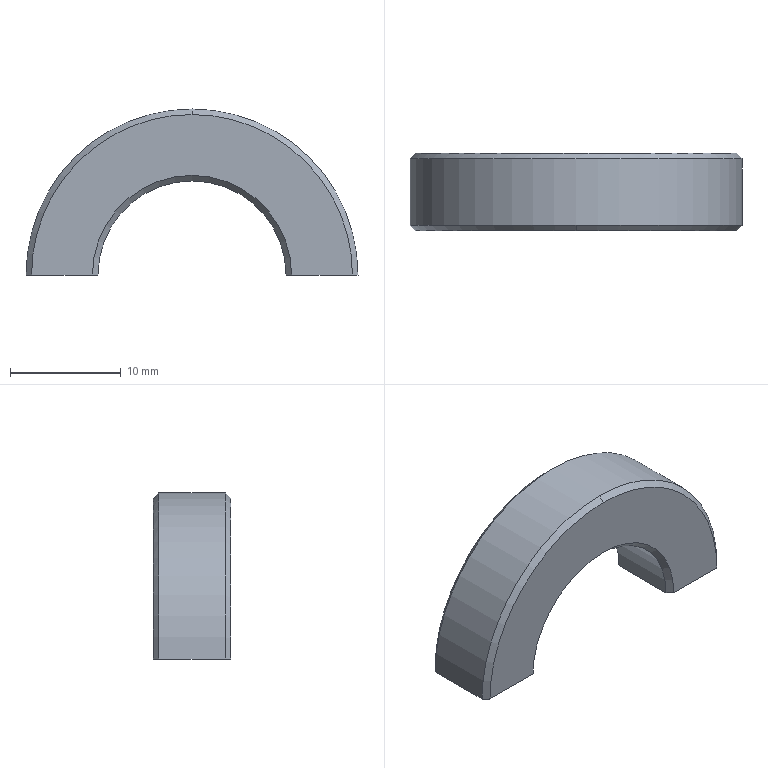Part | STEP file | 6903 ZZ | 1 solid | 12 faces | box 30 x 7 x 15 mm | volume 1661 mm3 | cone 6 | plane 4 | cylinder 2 | commonest cylinder face diameters 17 x1 30 x1
STEP:
#1=CARTESIAN_POINT('',(0.,0.,0.));
#2=DIRECTION('',(0.,0.,1.));
#3=DIRECTION('',(1.,0.,0.));
#4=AXIS2_PLACEMENT_3D('',#1,#2,#3);
#5=CARTESIAN_POINT('',(8.5,6.5,0.));
#6=VERTEX_POINT('',#5);
#7=CARTESIAN_POINT('',(9.,7.,0.));
#8=VERTEX_POINT('',#7);
#9=CARTESIAN_POINT('',(0.,-2.,0.));
#10=DIRECTION('',(0.7071,0.7071,0.));
#11=VECTOR('',#10,1.);
#12=LINE('',#9,#11);
#13=CARTESIAN_POINT('',(0.,6.5,0.));
#14=DIRECTION('',(0.,1.,0.));
#15=DIRECTION('',(0.,0.,1.));
#16=AXIS2_PLACEMENT_3D('',#13,#14,#15);
#17=CONICAL_SURFACE('',#16,8.5,0.7854);
#18=CARTESIAN_POINT('',(1.571,-8.5));
#19=DIRECTION('',(0.,1.));
#20=VECTOR('',#19,1.);
#21=LINE('',#18,#20);
#22=(GEOMETRIC_REPRESENTATION_CONTEXT(2)PARAMETRIC_REPRESENTATION_CONTEXT()REPRESENTATION_CONTEXT('',''));
#23=DEFINITIONAL_REPRESENTATION('',(#21),#22);
#24=PCURVE('',#17,#23);
#25=CARTESIAN_POINT('',(120.,-45.57,0.));
#26=DIRECTION('',(0.,0.,1.));
#27=DIRECTION('',(1.,0.,0.));
#28=AXIS2_PLACEMENT_3D('',#25,#26,#27);
#29=PLANE('',#28);
#30=CARTESIAN_POINT('',(-120.,43.57));
#31=DIRECTION('',(0.7071,0.7071));
#32=VECTOR('',#31,1.);
#33=LINE('',#30,#32);
#34=(GEOMETRIC_REPRESENTATION_CONTEXT(2)PARAMETRIC_REPRESENTATION_CONTEXT()REPRESENTATION_CONTEXT('',''));
#35=DEFINITIONAL_REPRESENTATION('',(#33),#34);
#36=PCURVE('',#29,#35);
#37=SURFACE_CURVE('',#12,(#24,#36),.PCURVE_S1.);
#38=EDGE_CURVE('',#6,#8,#37,.T.);
#39=ORIENTED_EDGE('',*,*,#38,.T.);
#40=CARTESIAN_POINT('',(0.,7.,9.));
#41=VERTEX_POINT('',#40);
#42=CARTESIAN_POINT('',(0.,7.,0.));
#43=DIRECTION('',(0.,-1.,0.));
#44=DIRECTION('',(0.,0.,1.));
#45=AXIS2_PLACEMENT_3D('',#42,#43,#44);
#46=CIRCLE('',#45,9.);
#47=CARTESIAN_POINT('',(6.283,0.5));
#48=DIRECTION('',(-1.,0.));
#49=VECTOR('',#48,1.);
#50=LINE('',#47,#49);
#51=(GEOMETRIC_REPRESENTATION_CONTEXT(2)PARAMETRIC_REPRESENTATION_CONTEXT()REPRESENTATION_CONTEXT('',''));
#52=DEFINITIONAL_REPRESENTATION('',(#50),#51);
#53=PCURVE('',#17,#52);
#54=CARTESIAN_POINT('',(0.,7.,0.));
#55=DIRECTION('',(0.,1.,0.));
#56=DIRECTION('',(0.,0.,1.));
#57=AXIS2_PLACEMENT_3D('',#54,#55,#56);
#58=PLANE('',#57);
#59=CARTESIAN_POINT('',(9.,0.));
#60=CARTESIAN_POINT('',(9.,-15.588));
#61=CARTESIAN_POINT('',(-4.5,-7.794));
#62=CARTESIAN_POINT('',(-18.,0.));
#63=CARTESIAN_POINT('',(-4.5,7.794));
#64=CARTESIAN_POINT('',(9.,15.588));
#65=CARTESIAN_POINT('',(9.,0.));
#66=(BOUNDED_CURVE()B_SPLINE_CURVE(2,(#59,#60,#61,#62,#63,#64,#65),.UNSPECIFIED.,.T.,.F.)B_SPLINE_CURVE_WITH_KNOTS((1,2,2,2,2,1),(-2.094,0.,2.094,4.189,6.283,8.378),.UNSPECIFIED.)CURVE()GEOMETRIC_REPRESENTATION_ITEM()RATIONAL_B_SPLINE_CURVE((1.,0.5,1.,0.5,1.,0.5,1.))REPRESENTATION_ITEM(''));
#67=(GEOMETRIC_REPRESENTATION_CONTEXT(2)PARAMETRIC_REPRESENTATION_CONTEXT()REPRESENTATION_CONTEXT('',''));
#68=DEFINITIONAL_REPRESENTATION('',(#66),#67);
#69=PCURVE('',#58,#68);
#70=SURFACE_CURVE('',#46,(#53,#69),.PCURVE_S1.);
#71=EDGE_CURVE('',#8,#41,#70,.T.);
#72=ORIENTED_EDGE('',*,*,#71,.T.);
#73=CARTESIAN_POINT('',(0.,6.5,8.5));
#74=VERTEX_POINT('',#73);
#75=CARTESIAN_POINT('',(0.,6.5,8.5));
#76=DIRECTION('',(0.,0.7071,0.7071));
#77=VECTOR('',#76,1.);
#78=LINE('',#75,#77);
#79=CARTESIAN_POINT('',(0.,0.));
#80=DIRECTION('',(0.,1.));
#81=VECTOR('',#80,1.);
#82=LINE('',#79,#81);
#83=(GEOMETRIC_REPRESENTATION_CONTEXT(2)PARAMETRIC_REPRESENTATION_CONTEXT()REPRESENTATION_CONTEXT('',''));
#84=DEFINITIONAL_REPRESENTATION('',(#82),#83);
#85=PCURVE('',#17,#84);
#86=CARTESIAN_POINT('',(0.,6.5,0.));
#87=DIRECTION('',(0.,1.,0.));
#88=DIRECTION('',(0.,0.,1.));
#89=AXIS2_PLACEMENT_3D('',#86,#87,#88);
#90=CONICAL_SURFACE('',#89,8.5,0.7854);
#91=CARTESIAN_POINT('',(6.283,0.));
#92=DIRECTION('',(0.,1.));
#93=VECTOR('',#92,1.);
#94=LINE('',#91,#93);
#95=(GEOMETRIC_REPRESENTATION_CONTEXT(2)PARAMETRIC_REPRESENTATION_CONTEXT()REPRESENTATION_CONTEXT('',''));
#96=DEFINITIONAL_REPRESENTATION('',(#94),#95);
#97=PCURVE('',#90,#96);
#98=SURFACE_CURVE('',#78,(#85,#97),.PCURVE_S1.);
#99=EDGE_CURVE('',#74,#41,#98,.T.);
#100=ORIENTED_EDGE('',*,*,#99,.F.);
#101=CARTESIAN_POINT('',(0.,6.5,0.));
#102=DIRECTION('',(0.,1.,0.));
#103=DIRECTION('',(0.,0.,1.));
#104=AXIS2_PLACEMENT_3D('',#101,#102,#103);
#105=CIRCLE('',#104,8.5);
#106=CARTESIAN_POINT('',(0.,0.));
#107=DIRECTION('',(1.,0.));
#108=VECTOR('',#107,1.);
#109=LINE('',#106,#108);
#110=(GEOMETRIC_REPRESENTATION_CONTEXT(2)PARAMETRIC_REPRESENTATION_CONTEXT()REPRESENTATION_CONTEXT('',''));
#111=DEFINITIONAL_REPRESENTATION('',(#109),#110);
#112=PCURVE('',#17,#111);
#113=CARTESIAN_POINT('',(0.,7.,0.));
#114=DIRECTION('',(0.,-1.,0.));
#115=DIRECTION('',(0.,0.,-1.));
#116=AXIS2_PLACEMENT_3D('',#113,#114,#115);
#117=CYLINDRICAL_SURFACE('',#116,8.5);
#118=CARTESIAN_POINT('',(3.142,0.5));
#119=DIRECTION('',(-1.,0.));
#120=VECTOR('',#119,1.);
#121=LINE('',#118,#120);
#122=(GEOMETRIC_REPRESENTATION_CONTEXT(2)PARAMETRIC_REPRESENTATION_CONTEXT()REPRESENTATION_CONTEXT('',''));
#123=DEFINITIONAL_REPRESENTATION('',(#121),#122);
#124=PCURVE('',#117,#123);
#125=SURFACE_CURVE('',#105,(#112,#124),.PCURVE_S1.);
#126=EDGE_CURVE('',#74,#6,#125,.T.);
#127=ORIENTED_EDGE('',*,*,#126,.T.);
#128=EDGE_LOOP('',(#39,#72,#100,#127));
#129=FACE_BOUND('',#128,.F.);
#130=ADVANCED_FACE('',(#129),#17,.F.);
#131=CARTESIAN_POINT('',(0.,0.,14.5));
#132=VERTEX_POINT('',#131);
#133=CARTESIAN_POINT('',(-14.5,0.,0.));
#134=VERTEX_POINT('',#133);
#135=CARTESIAN_POINT('',(0.,0.,0.));
#136=DIRECTION('',(0.,-1.,0.));
#137=DIRECTION('',(0.,0.,1.));
#138=AXIS2_PLACEMENT_3D('',#135,#136,#137);
#139=CIRCLE('',#138,14.5);
#140=CARTESIAN_POINT('',(0.,0.5,0.));
#141=DIRECTION('',(0.,1.,0.));
#142=DIRECTION('',(0.,0.,1.));
#143=AXIS2_PLACEMENT_3D('',#140,#141,#142);
#144=CONICAL_SURFACE('',#143,15.,0.7854);
#145=CARTESIAN_POINT('',(6.283,-0.5));
#146=DIRECTION('',(-1.,0.));
#147=VECTOR('',#146,1.);
#148=LINE('',#145,#147);
#149=(GEOMETRIC_REPRESENTATION_CONTEXT(2)PARAMETRIC_REPRESENTATION_CONTEXT()REPRESENTATION_CONTEXT('',''));
#150=DEFINITIONAL_REPRESENTATION('',(#148),#149);
#151=PCURVE('',#144,#150);
#152=CARTESIAN_POINT('',(0.,0.,0.));
#153=DIRECTION('',(0.,1.,0.));
#154=DIRECTION('',(0.,0.,1.));
#155=AXIS2_PLACEMENT_3D('',#152,#153,#154);
#156=PLANE('',#155);
#157=CARTESIAN_POINT('',(14.5,0.));
#158=CARTESIAN_POINT('',(14.5,-25.115));
#159=CARTESIAN_POINT('',(-7.25,-12.557));
#160=CARTESIAN_POINT('',(-29.,0.));
#161=CARTESIAN_POINT('',(-7.25,12.557));
#162=CARTESIAN_POINT('',(14.5,25.115));
#163=CARTESIAN_POINT('',(14.5,0.));
#164=(BOUNDED_CURVE()B_SPLINE_CURVE(2,(#157,#158,#159,#160,#161,#162,#163),.UNSPECIFIED.,.T.,.F.)B_SPLINE_CURVE_WITH_KNOTS((1,2,2,2,2,1),(-2.094,0.,2.094,4.189,6.283,8.378),.UNSPECIFIED.)CURVE()GEOMETRIC_REPRESENTATION_ITEM()RATIONAL_B_SPLINE_CURVE((1.,0.5,1.,0.5,1.,0.5,1.))REPRESENTATION_ITEM(''));
#165=(GEOMETRIC_REPRESENTATION_CONTEXT(2)PARAMETRIC_REPRESENTATION_CONTEXT()REPRESENTATION_CONTEXT('',''));
#166=DEFINITIONAL_REPRESENTATION('',(#164),#165);
#167=PCURVE('',#156,#166);
#168=SURFACE_CURVE('',#139,(#151,#167),.PCURVE_S1.);
#169=EDGE_CURVE('',#132,#134,#168,.T.);
#170=ORIENTED_EDGE('',*,*,#169,.F.);
#171=CARTESIAN_POINT('',(0.,0.5,15.));
#172=VERTEX_POINT('',#171);
#173=CARTESIAN_POINT('',(0.,0.5,15.));
#174=DIRECTION('',(0.,0.7071,0.7071));
#175=VECTOR('',#174,1.);
#176=LINE('',#173,#175);
#177=CARTESIAN_POINT('',(6.283,0.));
#178=DIRECTION('',(0.,1.));
#179=VECTOR('',#178,1.);
#180=LINE('',#177,#179);
#181=(GEOMETRIC_REPRESENTATION_CONTEXT(2)PARAMETRIC_REPRESENTATION_CONTEXT()REPRESENTATION_CONTEXT('',''));
#182=DEFINITIONAL_REPRESENTATION('',(#180),#181);
#183=PCURVE('',#144,#182);
#184=CARTESIAN_POINT('',(0.,0.5,0.));
#185=DIRECTION('',(0.,1.,0.));
#186=DIRECTION('',(0.,0.,1.));
#187=AXIS2_PLACEMENT_3D('',#184,#185,#186);
#188=CONICAL_SURFACE('',#187,15.,0.7854);
#189=CARTESIAN_POINT('',(0.,0.));
#190=DIRECTION('',(0.,1.));
#191=VECTOR('',#190,1.);
#192=LINE('',#189,#191);
#193=(GEOMETRIC_REPRESENTATION_CONTEXT(2)PARAMETRIC_REPRESENTATION_CONTEXT()REPRESENTATION_CONTEXT('',''));
#194=DEFINITIONAL_REPRESENTATION('',(#192),#193);
#195=PCURVE('',#188,#194);
#196=SURFACE_CURVE('',#176,(#183,#195),.PCURVE_S1.);
#197=EDGE_CURVE('',#132,#172,#196,.T.);
#198=ORIENTED_EDGE('',*,*,#197,.T.);
#199=CARTESIAN_POINT('',(-15.,0.5,0.));
#200=VERTEX_POINT('',#199);
#201=CARTESIAN_POINT('',(0.,0.5,0.));
#202=DIRECTION('',(0.,1.,0.));
#203=DIRECTION('',(0.,0.,1.));
#204=AXIS2_PLACEMENT_3D('',#201,#202,#203);
#205=CIRCLE('',#204,15.);
#206=CARTESIAN_POINT('',(0.,0.));
#207=DIRECTION('',(1.,0.));
#208=VECTOR('',#207,1.);
#209=LINE('',#206,#208);
#210=(GEOMETRIC_REPRESENTATION_CONTEXT(2)PARAMETRIC_REPRESENTATION_CONTEXT()REPRESENTATION_CONTEXT('',''));
#211=DEFINITIONAL_REPRESENTATION('',(#209),#210);
#212=PCURVE('',#144,#211);
#213=CARTESIAN_POINT('',(0.,7.,0.));
#214=DIRECTION('',(0.,-1.,0.));
#215=DIRECTION('',(0.,0.,-1.));
#216=AXIS2_PLACEMENT_3D('',#213,#214,#215);
#217=CYLINDRICAL_SURFACE('',#216,15.);
#218=CARTESIAN_POINT('',(9.425,6.5));
#219=DIRECTION('',(-1.,0.));
#220=VECTOR('',#219,1.);
#221=LINE('',#218,#220);
#222=(GEOMETRIC_REPRESENTATION_CONTEXT(2)PARAMETRIC_REPRESENTATION_CONTEXT()REPRESENTATION_CONTEXT('',''));
#223=DEFINITIONAL_REPRESENTATION('',(#221),#222);
#224=PCURVE('',#217,#223);
#225=SURFACE_CURVE('',#205,(#212,#224),.PCURVE_S1.);
#226=EDGE_CURVE('',#200,#172,#225,.T.);
#227=ORIENTED_EDGE('',*,*,#226,.F.);
#228=CARTESIAN_POINT('',(0.,-14.5,0.));
#229=DIRECTION('',(-0.7071,0.7071,0.));
#230=VECTOR('',#229,1.);
#231=LINE('',#228,#230);
#232=CARTESIAN_POINT('',(4.712,-15.));
#233=DIRECTION('',(0.,1.));
#234=VECTOR('',#233,1.);
#235=LINE('',#232,#234);
#236=(GEOMETRIC_REPRESENTATION_CONTEXT(2)PARAMETRIC_REPRESENTATION_CONTEXT()REPRESENTATION_CONTEXT('',''));
#237=DEFINITIONAL_REPRESENTATION('',(#235),#236);
#238=PCURVE('',#144,#237);
#239=CARTESIAN_POINT('',(120.,-45.57,0.));
#240=DIRECTION('',(0.,0.,1.));
#241=DIRECTION('',(1.,0.,0.));
#242=AXIS2_PLACEMENT_3D('',#239,#240,#241);
#243=PLANE('',#242);
#244=CARTESIAN_POINT('',(-120.,31.07));
#245=DIRECTION('',(-0.7071,0.7071));
#246=VECTOR('',#245,1.);
#247=LINE('',#244,#246);
#248=(GEOMETRIC_REPRESENTATION_CONTEXT(2)PARAMETRIC_REPRESENTATION_CONTEXT()REPRESENTATION_CONTEXT('',''));
#249=DEFINITIONAL_REPRESENTATION('',(#247),#248);
#250=PCURVE('',#243,#249);
#251=SURFACE_CURVE('',#231,(#238,#250),.PCURVE_S1.);
#252=EDGE_CURVE('',#134,#200,#251,.T.);
#253=ORIENTED_EDGE('',*,*,#252,.F.);
#254=EDGE_LOOP('',(#170,#198,#227,#253));
#255=FACE_BOUND('',#254,.T.);
#256=ADVANCED_FACE('',(#255),#144,.T.);
#257=CARTESIAN_POINT('',(-14.5,7.,0.));
#258=VERTEX_POINT('',#257);
#259=CARTESIAN_POINT('',(-9.,7.,0.));
#260=VERTEX_POINT('',#259);
#261=CARTESIAN_POINT('',(0.,7.,0.));
#262=DIRECTION('',(1.,0.,0.));
#263=VECTOR('',#262,1.);
#264=LINE('',#261,#263);
#265=CARTESIAN_POINT('',(0.,0.));
#266=DIRECTION('',(0.,1.));
#267=VECTOR('',#266,1.);
#268=LINE('',#265,#267);
#269=(GEOMETRIC_REPRESENTATION_CONTEXT(2)PARAMETRIC_REPRESENTATION_CONTEXT()REPRESENTATION_CONTEXT('',''));
#270=DEFINITIONAL_REPRESENTATION('',(#268),#269);
#271=PCURVE('',#58,#270);
#272=CARTESIAN_POINT('',(-120.,52.57));
#273=DIRECTION('',(1.,0.));
#274=VECTOR('',#273,1.);
#275=LINE('',#272,#274);
#276=(GEOMETRIC_REPRESENTATION_CONTEXT(2)PARAMETRIC_REPRESENTATION_CONTEXT()REPRESENTATION_CONTEXT('',''));
#277=DEFINITIONAL_REPRESENTATION('',(#275),#276);
#278=PCURVE('',#243,#277);
#279=SURFACE_CURVE('',#264,(#271,#278),.PCURVE_S1.);
#280=EDGE_CURVE('',#258,#260,#279,.T.);
#281=ORIENTED_EDGE('',*,*,#280,.F.);
#282=CARTESIAN_POINT('',(14.5,7.,0.));
#283=VERTEX_POINT('',#282);
#284=CARTESIAN_POINT('',(0.,7.,0.));
#285=DIRECTION('',(0.,1.,0.));
#286=DIRECTION('',(0.,0.,1.));
#287=AXIS2_PLACEMENT_3D('',#284,#285,#286);
#288=CIRCLE('',#287,14.5);
#289=CARTESIAN_POINT('',(0.,0.));
#290=DIRECTION('',(1.,0.));
#291=AXIS2_PLACEMENT_2D('',#289,#290);
#292=CIRCLE('',#291,14.5);
#293=(GEOMETRIC_REPRESENTATION_CONTEXT(2)PARAMETRIC_REPRESENTATION_CONTEXT()REPRESENTATION_CONTEXT('',''));
#294=DEFINITIONAL_REPRESENTATION('',(#292),#293);
#295=PCURVE('',#58,#294);
#296=CARTESIAN_POINT('',(0.,7.,0.));
#297=DIRECTION('',(0.,-1.,0.));
#298=DIRECTION('',(0.,0.,-1.));
#299=AXIS2_PLACEMENT_3D('',#296,#297,#298);
#300=CONICAL_SURFACE('',#299,14.5,0.7854);
#301=CARTESIAN_POINT('',(9.425,0.));
#302=DIRECTION('',(-1.,0.));
#303=VECTOR('',#302,1.);
#304=LINE('',#301,#303);
#305=(GEOMETRIC_REPRESENTATION_CONTEXT(2)PARAMETRIC_REPRESENTATION_CONTEXT()REPRESENTATION_CONTEXT('',''));
#306=DEFINITIONAL_REPRESENTATION('',(#304),#305);
#307=PCURVE('',#300,#306);
#308=SURFACE_CURVE('',#288,(#295,#307),.PCURVE_S1.);
#309=EDGE_CURVE('',#258,#283,#308,.T.);
#310=ORIENTED_EDGE('',*,*,#309,.T.);
#311=CARTESIAN_POINT('',(0.,7.,0.));
#312=DIRECTION('',(1.,0.,0.));
#313=VECTOR('',#312,1.);
#314=LINE('',#311,#313);
#315=CARTESIAN_POINT('',(0.,0.));
#316=DIRECTION('',(0.,1.));
#317=VECTOR('',#316,1.);
#318=LINE('',#315,#317);
#319=(GEOMETRIC_REPRESENTATION_CONTEXT(2)PARAMETRIC_REPRESENTATION_CONTEXT()REPRESENTATION_CONTEXT('',''));
#320=DEFINITIONAL_REPRESENTATION('',(#318),#319);
#321=PCURVE('',#58,#320);
#322=CARTESIAN_POINT('',(-120.,52.57));
#323=DIRECTION('',(1.,0.));
#324=VECTOR('',#323,1.);
#325=LINE('',#322,#324);
#326=(GEOMETRIC_REPRESENTATION_CONTEXT(2)PARAMETRIC_REPRESENTATION_CONTEXT()REPRESENTATION_CONTEXT('',''));
#327=DEFINITIONAL_REPRESENTATION('',(#325),#326);
#328=PCURVE('',#29,#327);
#329=SURFACE_CURVE('',#314,(#321,#328),.PCURVE_S1.);
#330=EDGE_CURVE('',#8,#283,#329,.T.);
#331=ORIENTED_EDGE('',*,*,#330,.F.);
#332=ORIENTED_EDGE('',*,*,#71,.T.);
#333=CARTESIAN_POINT('',(0.,7.,0.));
#334=DIRECTION('',(0.,-1.,0.));
#335=DIRECTION('',(0.,0.,1.));
#336=AXIS2_PLACEMENT_3D('',#333,#334,#335);
#337=CIRCLE('',#336,9.);
#338=CARTESIAN_POINT('',(9.,0.));
#339=CARTESIAN_POINT('',(9.,-15.588));
#340=CARTESIAN_POINT('',(-4.5,-7.794));
#341=CARTESIAN_POINT('',(-18.,0.));
#342=CARTESIAN_POINT('',(-4.5,7.794));
#343=CARTESIAN_POINT('',(9.,15.588));
#344=CARTESIAN_POINT('',(9.,0.));
#345=(BOUNDED_CURVE()B_SPLINE_CURVE(2,(#338,#339,#340,#341,#342,#343,#344),.UNSPECIFIED.,.T.,.F.)B_SPLINE_CURVE_WITH_KNOTS((1,2,2,2,2,1),(-2.094,0.,2.094,4.189,6.283,8.378),.UNSPECIFIED.)CURVE()GEOMETRIC_REPRESENTATION_ITEM()RATIONAL_B_SPLINE_CURVE((1.,0.5,1.,0.5,1.,0.5,1.))REPRESENTATION_ITEM(''));
#346=(GEOMETRIC_REPRESENTATION_CONTEXT(2)PARAMETRIC_REPRESENTATION_CONTEXT()REPRESENTATION_CONTEXT('',''));
#347=DEFINITIONAL_REPRESENTATION('',(#345),#346);
#348=PCURVE('',#58,#347);
#349=CARTESIAN_POINT('',(6.283,0.5));
#350=DIRECTION('',(-1.,0.));
#351=VECTOR('',#350,1.);
#352=LINE('',#349,#351);
#353=(GEOMETRIC_REPRESENTATION_CONTEXT(2)PARAMETRIC_REPRESENTATION_CONTEXT()REPRESENTATION_CONTEXT('',''));
#354=DEFINITIONAL_REPRESENTATION('',(#352),#353);
#355=PCURVE('',#90,#354);
#356=SURFACE_CURVE('',#337,(#348,#355),.PCURVE_S1.);
#357=EDGE_CURVE('',#41,#260,#356,.T.);
#358=ORIENTED_EDGE('',*,*,#357,.T.);
#359=EDGE_LOOP('',(#281,#310,#331,#332,#358));
#360=FACE_BOUND('',#359,.T.);
#361=ADVANCED_FACE('',(#360),#58,.T.);
#362=CARTESIAN_POINT('',(14.5,0.,0.));
#363=VERTEX_POINT('',#362);
#364=CARTESIAN_POINT('',(0.,0.,0.));
#365=DIRECTION('',(0.,-1.,0.));
#366=DIRECTION('',(0.,0.,1.));
#367=AXIS2_PLACEMENT_3D('',#364,#365,#366);
#368=CIRCLE('',#367,14.5);
#369=CARTESIAN_POINT('',(14.5,0.));
#370=CARTESIAN_POINT('',(14.5,-25.115));
#371=CARTESIAN_POINT('',(-7.25,-12.557));
#372=CARTESIAN_POINT('',(-29.,0.));
#373=CARTESIAN_POINT('',(-7.25,12.557));
#374=CARTESIAN_POINT('',(14.5,25.115));
#375=CARTESIAN_POINT('',(14.5,0.));
#376=(BOUNDED_CURVE()B_SPLINE_CURVE(2,(#369,#370,#371,#372,#373,#374,#375),.UNSPECIFIED.,.T.,.F.)B_SPLINE_CURVE_WITH_KNOTS((1,2,2,2,2,1),(-2.094,0.,2.094,4.189,6.283,8.378),.UNSPECIFIED.)CURVE()GEOMETRIC_REPRESENTATION_ITEM()RATIONAL_B_SPLINE_CURVE((1.,0.5,1.,0.5,1.,0.5,1.))REPRESENTATION_ITEM(''));
#377=(GEOMETRIC_REPRESENTATION_CONTEXT(2)PARAMETRIC_REPRESENTATION_CONTEXT()REPRESENTATION_CONTEXT('',''));
#378=DEFINITIONAL_REPRESENTATION('',(#376),#377);
#379=PCURVE('',#156,#378);
#380=CARTESIAN_POINT('',(6.283,-0.5));
#381=DIRECTION('',(-1.,0.));
#382=VECTOR('',#381,1.);
#383=LINE('',#380,#382);
#384=(GEOMETRIC_REPRESENTATION_CONTEXT(2)PARAMETRIC_REPRESENTATION_CONTEXT()REPRESENTATION_CONTEXT('',''));
#385=DEFINITIONAL_REPRESENTATION('',(#383),#384);
#386=PCURVE('',#188,#385);
#387=SURFACE_CURVE('',#368,(#379,#386),.PCURVE_S1.);
#388=EDGE_CURVE('',#363,#132,#387,.T.);
#389=ORIENTED_EDGE('',*,*,#388,.T.);
#390=ORIENTED_EDGE('',*,*,#169,.T.);
#391=CARTESIAN_POINT('',(-9.,0.,0.));
#392=VERTEX_POINT('',#391);
#393=CARTESIAN_POINT('',(0.,0.,0.));
#394=DIRECTION('',(1.,0.,0.));
#395=VECTOR('',#394,1.);
#396=LINE('',#393,#395);
#397=CARTESIAN_POINT('',(0.,0.));
#398=DIRECTION('',(0.,1.));
#399=VECTOR('',#398,1.);
#400=LINE('',#397,#399);
#401=(GEOMETRIC_REPRESENTATION_CONTEXT(2)PARAMETRIC_REPRESENTATION_CONTEXT()REPRESENTATION_CONTEXT('',''));
#402=DEFINITIONAL_REPRESENTATION('',(#400),#401);
#403=PCURVE('',#156,#402);
#404=CARTESIAN_POINT('',(-120.,45.57));
#405=DIRECTION('',(1.,0.));
#406=VECTOR('',#405,1.);
#407=LINE('',#404,#406);
#408=(GEOMETRIC_REPRESENTATION_CONTEXT(2)PARAMETRIC_REPRESENTATION_CONTEXT()REPRESENTATION_CONTEXT('',''));
#409=DEFINITIONAL_REPRESENTATION('',(#407),#408);
#410=PCURVE('',#243,#409);
#411=SURFACE_CURVE('',#396,(#403,#410),.PCURVE_S1.);
#412=EDGE_CURVE('',#134,#392,#411,.T.);
#413=ORIENTED_EDGE('',*,*,#412,.T.);
#414=CARTESIAN_POINT('',(9.,0.,0.));
#415=VERTEX_POINT('',#414);
#416=CARTESIAN_POINT('',(0.,0.,0.));
#417=DIRECTION('',(0.,1.,0.));
#418=DIRECTION('',(0.,0.,1.));
#419=AXIS2_PLACEMENT_3D('',#416,#417,#418);
#420=CIRCLE('',#419,9.);
#421=CARTESIAN_POINT('',(0.,0.));
#422=DIRECTION('',(1.,0.));
#423=AXIS2_PLACEMENT_2D('',#421,#422);
#424=CIRCLE('',#423,9.);
#425=(GEOMETRIC_REPRESENTATION_CONTEXT(2)PARAMETRIC_REPRESENTATION_CONTEXT()REPRESENTATION_CONTEXT('',''));
#426=DEFINITIONAL_REPRESENTATION('',(#424),#425);
#427=PCURVE('',#156,#426);
#428=CARTESIAN_POINT('',(0.,0.,0.));
#429=DIRECTION('',(0.,-1.,0.));
#430=DIRECTION('',(0.,0.,-1.));
#431=AXIS2_PLACEMENT_3D('',#428,#429,#430);
#432=CONICAL_SURFACE('',#431,9.,0.7854);
#433=CARTESIAN_POINT('',(9.425,0.));
#434=DIRECTION('',(-1.,0.));
#435=VECTOR('',#434,1.);
#436=LINE('',#433,#435);
#437=(GEOMETRIC_REPRESENTATION_CONTEXT(2)PARAMETRIC_REPRESENTATION_CONTEXT()REPRESENTATION_CONTEXT('',''));
#438=DEFINITIONAL_REPRESENTATION('',(#436),#437);
#439=PCURVE('',#432,#438);
#440=SURFACE_CURVE('',#420,(#427,#439),.PCURVE_S1.);
#441=EDGE_CURVE('',#392,#415,#440,.T.);
#442=ORIENTED_EDGE('',*,*,#441,.T.);
#443=CARTESIAN_POINT('',(0.,0.,0.));
#444=DIRECTION('',(1.,0.,0.));
#445=VECTOR('',#444,1.);
#446=LINE('',#443,#445);
#447=CARTESIAN_POINT('',(0.,0.));
#448=DIRECTION('',(0.,1.));
#449=VECTOR('',#448,1.);
#450=LINE('',#447,#449);
#451=(GEOMETRIC_REPRESENTATION_CONTEXT(2)PARAMETRIC_REPRESENTATION_CONTEXT()REPRESENTATION_CONTEXT('',''));
#452=DEFINITIONAL_REPRESENTATION('',(#450),#451);
#453=PCURVE('',#156,#452);
#454=CARTESIAN_POINT('',(-120.,45.57));
#455=DIRECTION('',(1.,0.));
#456=VECTOR('',#455,1.);
#457=LINE('',#454,#456);
#458=(GEOMETRIC_REPRESENTATION_CONTEXT(2)PARAMETRIC_REPRESENTATION_CONTEXT()REPRESENTATION_CONTEXT('',''));
#459=DEFINITIONAL_REPRESENTATION('',(#457),#458);
#460=PCURVE('',#29,#459);
#461=SURFACE_CURVE('',#446,(#453,#460),.PCURVE_S1.);
#462=EDGE_CURVE('',#415,#363,#461,.T.);
#463=ORIENTED_EDGE('',*,*,#462,.T.);
#464=EDGE_LOOP('',(#389,#390,#413,#442,#463));
#465=FACE_BOUND('',#464,.T.);
#466=ADVANCED_FACE('',(#465),#156,.F.);
#467=CARTESIAN_POINT('',(15.,6.5,0.));
#468=VERTEX_POINT('',#467);
#469=CARTESIAN_POINT('',(-15.,6.5,0.));
#470=VERTEX_POINT('',#469);
#471=CARTESIAN_POINT('',(0.,6.5,0.));
#472=DIRECTION('',(0.,-1.,0.));
#473=DIRECTION('',(0.,0.,1.));
#474=AXIS2_PLACEMENT_3D('',#471,#472,#473);
#475=CIRCLE('',#474,15.);
#476=CARTESIAN_POINT('',(-3.142,0.5));
#477=DIRECTION('',(1.,0.));
#478=VECTOR('',#477,1.);
#479=LINE('',#476,#478);
#480=(GEOMETRIC_REPRESENTATION_CONTEXT(2)PARAMETRIC_REPRESENTATION_CONTEXT()REPRESENTATION_CONTEXT('',''));
#481=DEFINITIONAL_REPRESENTATION('',(#479),#480);
#482=PCURVE('',#217,#481);
#483=CARTESIAN_POINT('',(-3.142,0.5));
#484=DIRECTION('',(1.,0.));
#485=VECTOR('',#484,1.);
#486=LINE('',#483,#485);
#487=(GEOMETRIC_REPRESENTATION_CONTEXT(2)PARAMETRIC_REPRESENTATION_CONTEXT()REPRESENTATION_CONTEXT('',''));
#488=DEFINITIONAL_REPRESENTATION('',(#486),#487);
#489=PCURVE('',#300,#488);
#490=SURFACE_CURVE('',#475,(#482,#489),.PCURVE_S1.);
#491=EDGE_CURVE('',#468,#470,#490,.T.);
#492=ORIENTED_EDGE('',*,*,#491,.T.);
#493=CARTESIAN_POINT('',(-15.,7.,0.));
#494=DIRECTION('',(0.,-1.,0.));
#495=VECTOR('',#494,1.);
#496=LINE('',#493,#495);
#497=CARTESIAN_POINT('',(4.712,0.));
#498=DIRECTION('',(0.,1.));
#499=VECTOR('',#498,1.);
#500=LINE('',#497,#499);
#501=(GEOMETRIC_REPRESENTATION_CONTEXT(2)PARAMETRIC_REPRESENTATION_CONTEXT()REPRESENTATION_CONTEXT('',''));
#502=DEFINITIONAL_REPRESENTATION('',(#500),#501);
#503=PCURVE('',#217,#502);
#504=CARTESIAN_POINT('',(-135.,52.57));
#505=DIRECTION('',(0.,-1.));
#506=VECTOR('',#505,1.);
#507=LINE('',#504,#506);
#508=(GEOMETRIC_REPRESENTATION_CONTEXT(2)PARAMETRIC_REPRESENTATION_CONTEXT()REPRESENTATION_CONTEXT('',''));
#509=DEFINITIONAL_REPRESENTATION('',(#507),#508);
#510=PCURVE('',#243,#509);
#511=SURFACE_CURVE('',#496,(#503,#510),.PCURVE_S1.);
#512=EDGE_CURVE('',#470,#200,#511,.T.);
#513=ORIENTED_EDGE('',*,*,#512,.T.);
#514=ORIENTED_EDGE('',*,*,#226,.T.);
#515=CARTESIAN_POINT('',(15.,0.5,0.));
#516=VERTEX_POINT('',#515);
#517=CARTESIAN_POINT('',(0.,0.5,0.));
#518=DIRECTION('',(0.,1.,0.));
#519=DIRECTION('',(0.,0.,1.));
#520=AXIS2_PLACEMENT_3D('',#517,#518,#519);
#521=CIRCLE('',#520,15.);
#522=CARTESIAN_POINT('',(3.142,6.5));
#523=DIRECTION('',(-1.,0.));
#524=VECTOR('',#523,1.);
#525=LINE('',#522,#524);
#526=(GEOMETRIC_REPRESENTATION_CONTEXT(2)PARAMETRIC_REPRESENTATION_CONTEXT()REPRESENTATION_CONTEXT('',''));
#527=DEFINITIONAL_REPRESENTATION('',(#525),#526);
#528=PCURVE('',#217,#527);
#529=CARTESIAN_POINT('',(0.,0.));
#530=DIRECTION('',(1.,0.));
#531=VECTOR('',#530,1.);
#532=LINE('',#529,#531);
#533=(GEOMETRIC_REPRESENTATION_CONTEXT(2)PARAMETRIC_REPRESENTATION_CONTEXT()REPRESENTATION_CONTEXT('',''));
#534=DEFINITIONAL_REPRESENTATION('',(#532),#533);
#535=PCURVE('',#188,#534);
#536=SURFACE_CURVE('',#521,(#528,#535),.PCURVE_S1.);
#537=EDGE_CURVE('',#172,#516,#536,.T.);
#538=ORIENTED_EDGE('',*,*,#537,.T.);
#539=CARTESIAN_POINT('',(15.,7.,0.));
#540=DIRECTION('',(0.,1.,0.));
#541=VECTOR('',#540,1.);
#542=LINE('',#539,#541);
#543=CARTESIAN_POINT('',(1.571,0.));
#544=DIRECTION('',(0.,-1.));
#545=VECTOR('',#544,1.);
#546=LINE('',#543,#545);
#547=(GEOMETRIC_REPRESENTATION_CONTEXT(2)PARAMETRIC_REPRESENTATION_CONTEXT()REPRESENTATION_CONTEXT('',''));
#548=DEFINITIONAL_REPRESENTATION('',(#546),#547);
#549=PCURVE('',#217,#548);
#550=CARTESIAN_POINT('',(-105.,52.57));
#551=DIRECTION('',(0.,1.));
#552=VECTOR('',#551,1.);
#553=LINE('',#550,#552);
#554=(GEOMETRIC_REPRESENTATION_CONTEXT(2)PARAMETRIC_REPRESENTATION_CONTEXT()REPRESENTATION_CONTEXT('',''));
#555=DEFINITIONAL_REPRESENTATION('',(#553),#554);
#556=PCURVE('',#29,#555);
#557=SURFACE_CURVE('',#542,(#549,#556),.PCURVE_S1.);
#558=EDGE_CURVE('',#516,#468,#557,.T.);
#559=ORIENTED_EDGE('',*,*,#558,.T.);
#560=EDGE_LOOP('',(#492,#513,#514,#538,#559));
#561=FACE_BOUND('',#560,.T.);
#562=ADVANCED_FACE('',(#561),#217,.T.);
#563=CARTESIAN_POINT('',(8.5,0.5,0.));
#564=VERTEX_POINT('',#563);
#565=CARTESIAN_POINT('',(-8.5,0.5,0.));
#566=VERTEX_POINT('',#565);
#567=CARTESIAN_POINT('',(0.,0.5,0.));
#568=DIRECTION('',(0.,-1.,0.));
#569=DIRECTION('',(0.,0.,1.));
#570=AXIS2_PLACEMENT_3D('',#567,#568,#569);
#571=CIRCLE('',#570,8.5);
#572=CARTESIAN_POINT('',(-3.142,6.5));
#573=DIRECTION('',(1.,0.));
#574=VECTOR('',#573,1.);
#575=LINE('',#572,#574);
#576=(GEOMETRIC_REPRESENTATION_CONTEXT(2)PARAMETRIC_REPRESENTATION_CONTEXT()REPRESENTATION_CONTEXT('',''));
#577=DEFINITIONAL_REPRESENTATION('',(#575),#576);
#578=PCURVE('',#117,#577);
#579=CARTESIAN_POINT('',(-3.142,-0.5));
#580=DIRECTION('',(1.,0.));
#581=VECTOR('',#580,1.);
#582=LINE('',#579,#581);
#583=(GEOMETRIC_REPRESENTATION_CONTEXT(2)PARAMETRIC_REPRESENTATION_CONTEXT()REPRESENTATION_CONTEXT('',''));
#584=DEFINITIONAL_REPRESENTATION('',(#582),#583);
#585=PCURVE('',#432,#584);
#586=SURFACE_CURVE('',#571,(#578,#585),.PCURVE_S1.);
#587=EDGE_CURVE('',#564,#566,#586,.T.);
#588=ORIENTED_EDGE('',*,*,#587,.F.);
#589=CARTESIAN_POINT('',(8.5,7.,0.));
#590=DIRECTION('',(0.,1.,0.));
#591=VECTOR('',#590,1.);
#592=LINE('',#589,#591);
#593=CARTESIAN_POINT('',(1.571,0.));
#594=DIRECTION('',(0.,-1.));
#595=VECTOR('',#594,1.);
#596=LINE('',#593,#595);
#597=(GEOMETRIC_REPRESENTATION_CONTEXT(2)PARAMETRIC_REPRESENTATION_CONTEXT()REPRESENTATION_CONTEXT('',''));
#598=DEFINITIONAL_REPRESENTATION('',(#596),#597);
#599=PCURVE('',#117,#598);
#600=CARTESIAN_POINT('',(-111.5,52.57));
#601=DIRECTION('',(0.,1.));
#602=VECTOR('',#601,1.);
#603=LINE('',#600,#602);
#604=(GEOMETRIC_REPRESENTATION_CONTEXT(2)PARAMETRIC_REPRESENTATION_CONTEXT()REPRESENTATION_CONTEXT('',''));
#605=DEFINITIONAL_REPRESENTATION('',(#603),#604);
#606=PCURVE('',#29,#605);
#607=SURFACE_CURVE('',#592,(#599,#606),.PCURVE_S1.);
#608=EDGE_CURVE('',#564,#6,#607,.T.);
#609=ORIENTED_EDGE('',*,*,#608,.T.);
#610=ORIENTED_EDGE('',*,*,#126,.F.);
#611=CARTESIAN_POINT('',(-8.5,6.5,0.));
#612=VERTEX_POINT('',#611);
#613=CARTESIAN_POINT('',(0.,6.5,0.));
#614=DIRECTION('',(0.,1.,0.));
#615=DIRECTION('',(0.,0.,1.));
#616=AXIS2_PLACEMENT_3D('',#613,#614,#615);
#617=CIRCLE('',#616,8.5);
#618=CARTESIAN_POINT('',(9.425,0.5));
#619=DIRECTION('',(-1.,0.));
#620=VECTOR('',#619,1.);
#621=LINE('',#618,#620);
#622=(GEOMETRIC_REPRESENTATION_CONTEXT(2)PARAMETRIC_REPRESENTATION_CONTEXT()REPRESENTATION_CONTEXT('',''));
#623=DEFINITIONAL_REPRESENTATION('',(#621),#622);
#624=PCURVE('',#117,#623);
#625=CARTESIAN_POINT('',(0.,0.));
#626=DIRECTION('',(1.,0.));
#627=VECTOR('',#626,1.);
#628=LINE('',#625,#627);
#629=(GEOMETRIC_REPRESENTATION_CONTEXT(2)PARAMETRIC_REPRESENTATION_CONTEXT()REPRESENTATION_CONTEXT('',''));
#630=DEFINITIONAL_REPRESENTATION('',(#628),#629);
#631=PCURVE('',#90,#630);
#632=SURFACE_CURVE('',#617,(#624,#631),.PCURVE_S1.);
#633=EDGE_CURVE('',#612,#74,#632,.T.);
#634=ORIENTED_EDGE('',*,*,#633,.F.);
#635=CARTESIAN_POINT('',(-8.5,7.,0.));
#636=DIRECTION('',(0.,-1.,0.));
#637=VECTOR('',#636,1.);
#638=LINE('',#635,#637);
#639=CARTESIAN_POINT('',(4.712,0.));
#640=DIRECTION('',(0.,1.));
#641=VECTOR('',#640,1.);
#642=LINE('',#639,#641);
#643=(GEOMETRIC_REPRESENTATION_CONTEXT(2)PARAMETRIC_REPRESENTATION_CONTEXT()REPRESENTATION_CONTEXT('',''));
#644=DEFINITIONAL_REPRESENTATION('',(#642),#643);
#645=PCURVE('',#117,#644);
#646=CARTESIAN_POINT('',(-128.5,52.57));
#647=DIRECTION('',(0.,-1.));
#648=VECTOR('',#647,1.);
#649=LINE('',#646,#648);
#650=(GEOMETRIC_REPRESENTATION_CONTEXT(2)PARAMETRIC_REPRESENTATION_CONTEXT()REPRESENTATION_CONTEXT('',''));
#651=DEFINITIONAL_REPRESENTATION('',(#649),#650);
#652=PCURVE('',#243,#651);
#653=SURFACE_CURVE('',#638,(#645,#652),.PCURVE_S1.);
#654=EDGE_CURVE('',#612,#566,#653,.T.);
#655=ORIENTED_EDGE('',*,*,#654,.T.);
#656=EDGE_LOOP('',(#588,#609,#610,#634,#655));
#657=FACE_BOUND('',#656,.F.);
#658=ADVANCED_FACE('',(#657),#117,.F.);
#659=ORIENTED_EDGE('',*,*,#197,.F.);
#660=ORIENTED_EDGE('',*,*,#388,.F.);
#661=CARTESIAN_POINT('',(0.,-14.5,0.));
#662=DIRECTION('',(-0.7071,-0.7071,0.));
#663=VECTOR('',#662,1.);
#664=LINE('',#661,#663);
#665=CARTESIAN_POINT('',(1.571,-15.));
#666=DIRECTION('',(0.,-1.));
#667=VECTOR('',#666,1.);
#668=LINE('',#665,#667);
#669=(GEOMETRIC_REPRESENTATION_CONTEXT(2)PARAMETRIC_REPRESENTATION_CONTEXT()REPRESENTATION_CONTEXT('',''));
#670=DEFINITIONAL_REPRESENTATION('',(#668),#669);
#671=PCURVE('',#188,#670);
#672=CARTESIAN_POINT('',(-120.,31.07));
#673=DIRECTION('',(-0.7071,-0.7071));
#674=VECTOR('',#673,1.);
#675=LINE('',#672,#674);
#676=(GEOMETRIC_REPRESENTATION_CONTEXT(2)PARAMETRIC_REPRESENTATION_CONTEXT()REPRESENTATION_CONTEXT('',''));
#677=DEFINITIONAL_REPRESENTATION('',(#675),#676);
#678=PCURVE('',#29,#677);
#679=SURFACE_CURVE('',#664,(#671,#678),.PCURVE_S1.);
#680=EDGE_CURVE('',#516,#363,#679,.T.);
#681=ORIENTED_EDGE('',*,*,#680,.F.);
#682=ORIENTED_EDGE('',*,*,#537,.F.);
#683=EDGE_LOOP('',(#659,#660,#681,#682));
#684=FACE_BOUND('',#683,.T.);
#685=ADVANCED_FACE('',(#684),#188,.T.);
#686=ORIENTED_EDGE('',*,*,#441,.T.);
#687=CARTESIAN_POINT('',(0.,9.,0.));
#688=DIRECTION('',(-0.7071,0.7071,0.));
#689=VECTOR('',#688,1.);
#690=LINE('',#687,#689);
#691=CARTESIAN_POINT('',(1.571,-9.));
#692=DIRECTION('',(0.,-1.));
#693=VECTOR('',#692,1.);
#694=LINE('',#691,#693);
#695=(GEOMETRIC_REPRESENTATION_CONTEXT(2)PARAMETRIC_REPRESENTATION_CONTEXT()REPRESENTATION_CONTEXT('',''));
#696=DEFINITIONAL_REPRESENTATION('',(#694),#695);
#697=PCURVE('',#432,#696);
#698=CARTESIAN_POINT('',(-120.,54.57));
#699=DIRECTION('',(-0.7071,0.7071));
#700=VECTOR('',#699,1.);
#701=LINE('',#698,#700);
#702=(GEOMETRIC_REPRESENTATION_CONTEXT(2)PARAMETRIC_REPRESENTATION_CONTEXT()REPRESENTATION_CONTEXT('',''));
#703=DEFINITIONAL_REPRESENTATION('',(#701),#702);
#704=PCURVE('',#29,#703);
#705=SURFACE_CURVE('',#690,(#697,#704),.PCURVE_S1.);
#706=EDGE_CURVE('',#415,#564,#705,.T.);
#707=ORIENTED_EDGE('',*,*,#706,.T.);
#708=ORIENTED_EDGE('',*,*,#587,.T.);
#709=CARTESIAN_POINT('',(0.,9.,0.));
#710=DIRECTION('',(-0.7071,-0.7071,0.));
#711=VECTOR('',#710,1.);
#712=LINE('',#709,#711);
#713=CARTESIAN_POINT('',(4.712,-9.));
#714=DIRECTION('',(0.,1.));
#715=VECTOR('',#714,1.);
#716=LINE('',#713,#715);
#717=(GEOMETRIC_REPRESENTATION_CONTEXT(2)PARAMETRIC_REPRESENTATION_CONTEXT()REPRESENTATION_CONTEXT('',''));
#718=DEFINITIONAL_REPRESENTATION('',(#716),#717);
#719=PCURVE('',#432,#718);
#720=CARTESIAN_POINT('',(-120.,54.57));
#721=DIRECTION('',(-0.7071,-0.7071));
#722=VECTOR('',#721,1.);
#723=LINE('',#720,#722);
#724=(GEOMETRIC_REPRESENTATION_CONTEXT(2)PARAMETRIC_REPRESENTATION_CONTEXT()REPRESENTATION_CONTEXT('',''));
#725=DEFINITIONAL_REPRESENTATION('',(#723),#724);
#726=PCURVE('',#243,#725);
#727=SURFACE_CURVE('',#712,(#719,#726),.PCURVE_S1.);
#728=EDGE_CURVE('',#566,#392,#727,.T.);
#729=ORIENTED_EDGE('',*,*,#728,.T.);
#730=EDGE_LOOP('',(#686,#707,#708,#729));
#731=FACE_BOUND('',#730,.F.);
#732=ADVANCED_FACE('',(#731),#432,.F.);
#733=CARTESIAN_POINT('',(0.,21.5,0.));
#734=DIRECTION('',(0.7071,0.7071,0.));
#735=VECTOR('',#734,1.);
#736=LINE('',#733,#735);
#737=CARTESIAN_POINT('',(4.712,-14.5));
#738=DIRECTION('',(0.,-1.));
#739=VECTOR('',#738,1.);
#740=LINE('',#737,#739);
#741=(GEOMETRIC_REPRESENTATION_CONTEXT(2)PARAMETRIC_REPRESENTATION_CONTEXT()REPRESENTATION_CONTEXT('',''));
#742=DEFINITIONAL_REPRESENTATION('',(#740),#741);
#743=PCURVE('',#300,#742);
#744=CARTESIAN_POINT('',(-120.,67.07));
#745=DIRECTION('',(0.7071,0.7071));
#746=VECTOR('',#745,1.);
#747=LINE('',#744,#746);
#748=(GEOMETRIC_REPRESENTATION_CONTEXT(2)PARAMETRIC_REPRESENTATION_CONTEXT()REPRESENTATION_CONTEXT('',''));
#749=DEFINITIONAL_REPRESENTATION('',(#747),#748);
#750=PCURVE('',#243,#749);
#751=SURFACE_CURVE('',#736,(#743,#750),.PCURVE_S1.);
#752=EDGE_CURVE('',#470,#258,#751,.T.);
#753=ORIENTED_EDGE('',*,*,#752,.F.);
#754=ORIENTED_EDGE('',*,*,#491,.F.);
#755=CARTESIAN_POINT('',(0.,21.5,0.));
#756=DIRECTION('',(0.7071,-0.7071,0.));
#757=VECTOR('',#756,1.);
#758=LINE('',#755,#757);
#759=CARTESIAN_POINT('',(1.571,-14.5));
#760=DIRECTION('',(0.,1.));
#761=VECTOR('',#760,1.);
#762=LINE('',#759,#761);
#763=(GEOMETRIC_REPRESENTATION_CONTEXT(2)PARAMETRIC_REPRESENTATION_CONTEXT()REPRESENTATION_CONTEXT('',''));
#764=DEFINITIONAL_REPRESENTATION('',(#762),#763);
#765=PCURVE('',#300,#764);
#766=CARTESIAN_POINT('',(-120.,67.07));
#767=DIRECTION('',(0.7071,-0.7071));
#768=VECTOR('',#767,1.);
#769=LINE('',#766,#768);
#770=(GEOMETRIC_REPRESENTATION_CONTEXT(2)PARAMETRIC_REPRESENTATION_CONTEXT()REPRESENTATION_CONTEXT('',''));
#771=DEFINITIONAL_REPRESENTATION('',(#769),#770);
#772=PCURVE('',#29,#771);
#773=SURFACE_CURVE('',#758,(#765,#772),.PCURVE_S1.);
#774=EDGE_CURVE('',#283,#468,#773,.T.);
#775=ORIENTED_EDGE('',*,*,#774,.F.);
#776=ORIENTED_EDGE('',*,*,#309,.F.);
#777=EDGE_LOOP('',(#753,#754,#775,#776));
#778=FACE_BOUND('',#777,.T.);
#779=ADVANCED_FACE('',(#778),#300,.T.);
#780=ORIENTED_EDGE('',*,*,#357,.T.);
#781=CARTESIAN_POINT('',(0.,-2.,0.));
#782=DIRECTION('',(0.7071,-0.7071,0.));
#783=VECTOR('',#782,1.);
#784=LINE('',#781,#783);
#785=CARTESIAN_POINT('',(4.712,-8.5));
#786=DIRECTION('',(0.,-1.));
#787=VECTOR('',#786,1.);
#788=LINE('',#785,#787);
#789=(GEOMETRIC_REPRESENTATION_CONTEXT(2)PARAMETRIC_REPRESENTATION_CONTEXT()REPRESENTATION_CONTEXT('',''));
#790=DEFINITIONAL_REPRESENTATION('',(#788),#789);
#791=PCURVE('',#90,#790);
#792=CARTESIAN_POINT('',(-120.,43.57));
#793=DIRECTION('',(0.7071,-0.7071));
#794=VECTOR('',#793,1.);
#795=LINE('',#792,#794);
#796=(GEOMETRIC_REPRESENTATION_CONTEXT(2)PARAMETRIC_REPRESENTATION_CONTEXT()REPRESENTATION_CONTEXT('',''));
#797=DEFINITIONAL_REPRESENTATION('',(#795),#796);
#798=PCURVE('',#243,#797);
#799=SURFACE_CURVE('',#784,(#791,#798),.PCURVE_S1.);
#800=EDGE_CURVE('',#260,#612,#799,.T.);
#801=ORIENTED_EDGE('',*,*,#800,.T.);
#802=ORIENTED_EDGE('',*,*,#633,.T.);
#803=ORIENTED_EDGE('',*,*,#99,.T.);
#804=EDGE_LOOP('',(#780,#801,#802,#803));
#805=FACE_BOUND('',#804,.F.);
#806=ADVANCED_FACE('',(#805),#90,.F.);
#807=ORIENTED_EDGE('',*,*,#252,.T.);
#808=ORIENTED_EDGE('',*,*,#512,.F.);
#809=ORIENTED_EDGE('',*,*,#752,.T.);
#810=ORIENTED_EDGE('',*,*,#280,.T.);
#811=ORIENTED_EDGE('',*,*,#800,.T.);
#812=ORIENTED_EDGE('',*,*,#654,.T.);
#813=ORIENTED_EDGE('',*,*,#728,.T.);
#814=ORIENTED_EDGE('',*,*,#412,.F.);
#815=EDGE_LOOP('',(#807,#808,#809,#810,#811,#812,#813,#814));
#816=FACE_BOUND('',#815,.T.);
#817=ADVANCED_FACE('',(#816),#243,.F.);
#818=ORIENTED_EDGE('',*,*,#680,.T.);
#819=ORIENTED_EDGE('',*,*,#462,.F.);
#820=ORIENTED_EDGE('',*,*,#706,.T.);
#821=ORIENTED_EDGE('',*,*,#608,.T.);
#822=ORIENTED_EDGE('',*,*,#38,.T.);
#823=ORIENTED_EDGE('',*,*,#330,.T.);
#824=ORIENTED_EDGE('',*,*,#774,.T.);
#825=ORIENTED_EDGE('',*,*,#558,.F.);
#826=EDGE_LOOP('',(#818,#819,#820,#821,#822,#823,#824,#825));
#827=FACE_BOUND('',#826,.T.);
#828=ADVANCED_FACE('',(#827),#29,.F.);
#829=CLOSED_SHELL('',(#130,#256,#361,#466,#562,#658,#685,#732,#779,#806,#817,#828));
#830=MANIFOLD_SOLID_BREP('',#829);
#831=(LENGTH_UNIT()NAMED_UNIT(*)SI_UNIT(.MILLI.,.METRE.));
#832=UNCERTAINTY_MEASURE_WITH_UNIT(LENGTH_MEASURE(0.0000001),#831,'','');
#833=(NAMED_UNIT(*)PLANE_ANGLE_UNIT()SI_UNIT($,.RADIAN.));
#834=(NAMED_UNIT(*)SI_UNIT($,.STERADIAN.)SOLID_ANGLE_UNIT());
#835=(GEOMETRIC_REPRESENTATION_CONTEXT(3)GLOBAL_UNCERTAINTY_ASSIGNED_CONTEXT((#832))GLOBAL_UNIT_ASSIGNED_CONTEXT((#831,#833,#834))REPRESENTATION_CONTEXT('',''));
#836=ADVANCED_BREP_SHAPE_REPRESENTATION('',(#4,#830),#835);